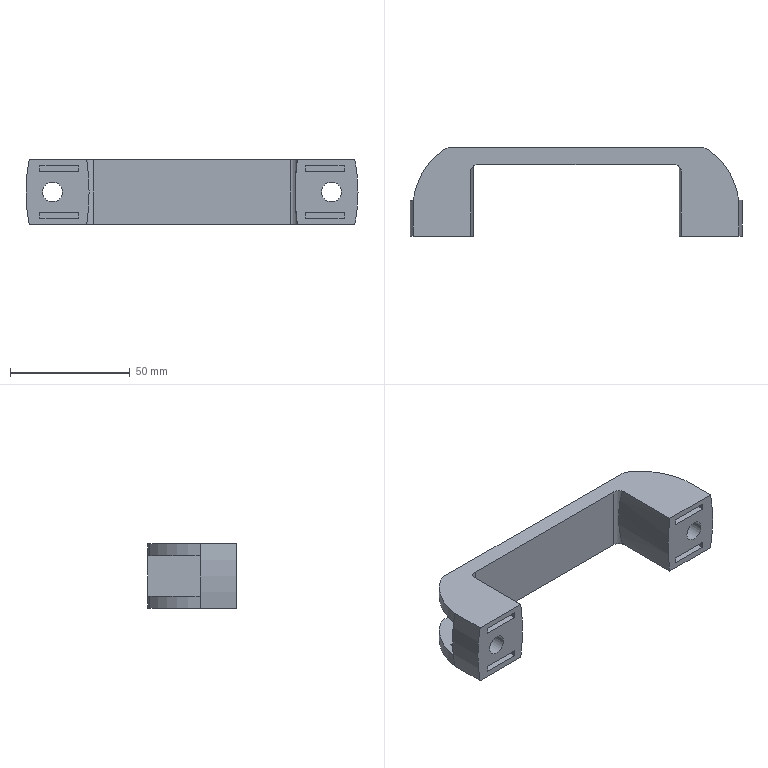Part | SolidWorks | features ICE 6, Extrusion 1 | 1 solid | 60 faces | box 138.654 x 37 x 27 mm | volume 43785 mm3 | plane 36 | cylinder 24 | commonest cylinder face diameters 8.2 x4 10 x4 13 x4 60 x4 138.654 x3 183.25 x3